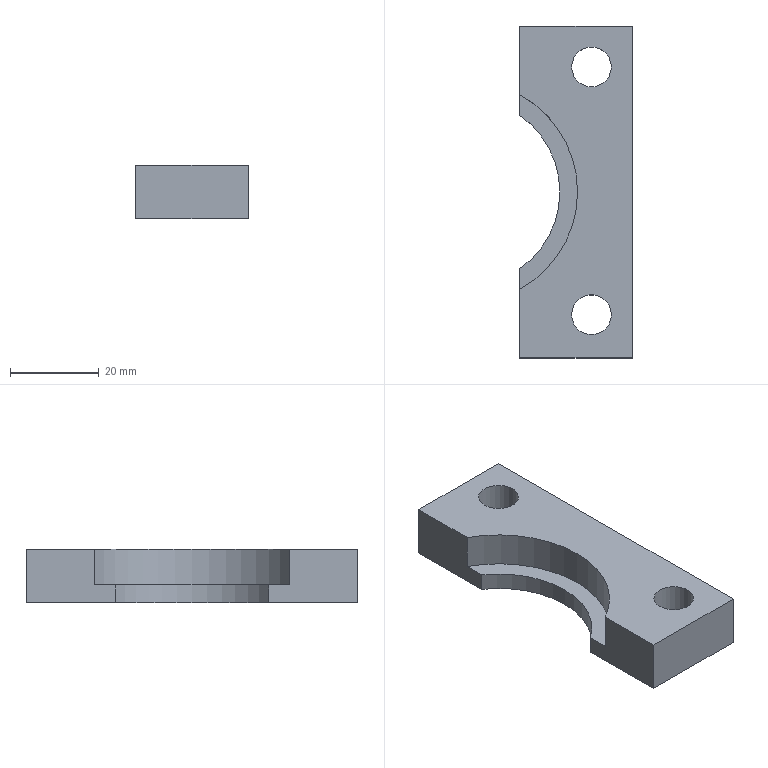Part | NX | features solid 2 | 1 solid | 12 faces | box 25.5 x 75 x 12 mm | volume 17248 mm3 | plane 8 | cylinder 4 | commonest cylinder face diameters 9 x2 42.2 x1 50.2 x1
STEP:
#1=CARTESIAN_POINT('',(772.5,172.5,250.));
#2=VERTEX_POINT('',#1);
#3=CARTESIAN_POINT('',(747.,172.5,250.));
#4=VERTEX_POINT('',#3);
#5=CARTESIAN_POINT('',(772.5,172.5,250.));
#6=DIRECTION('',(-1.,0.,0.));
#7=VECTOR('',#6,1000.);
#8=LINE('',#5,#7);
#9=EDGE_CURVE('',#2,#4,#8,.T.);
#10=ORIENTED_EDGE('',*,*,#9,.T.);
#11=CARTESIAN_POINT('',(747.,172.5,238.));
#12=VERTEX_POINT('',#11);
#13=CARTESIAN_POINT('',(747.,172.5,242.));
#14=DIRECTION('',(0.,0.,1.));
#15=VECTOR('',#14,1000.);
#16=LINE('',#13,#15);
#17=EDGE_CURVE('',#12,#4,#16,.T.);
#18=ORIENTED_EDGE('',*,*,#17,.F.);
#19=CARTESIAN_POINT('',(772.5,172.5,238.));
#20=VERTEX_POINT('',#19);
#21=CARTESIAN_POINT('',(772.5,172.5,238.));
#22=DIRECTION('',(-1.,0.,0.));
#23=VECTOR('',#22,1000.);
#24=LINE('',#21,#23);
#25=EDGE_CURVE('',#20,#12,#24,.T.);
#26=ORIENTED_EDGE('',*,*,#25,.F.);
#27=CARTESIAN_POINT('',(772.5,172.5,242.));
#28=DIRECTION('',(0.,0.,1.));
#29=VECTOR('',#28,1000.);
#30=LINE('',#27,#29);
#31=EDGE_CURVE('',#20,#2,#30,.T.);
#32=ORIENTED_EDGE('',*,*,#31,.T.);
#33=EDGE_LOOP('',(#10,#18,#26,#32));
#34=FACE_BOUND('',#33,.T.);
#35=CARTESIAN_POINT('',(772.5,172.5,242.));
#36=DIRECTION('',(0.,1.,0.));
#37=DIRECTION('',(0.,0.,1.));
#38=AXIS2_PLACEMENT_3D('',#35,#36,#37);
#39=PLANE('',#38);
#40=ADVANCED_FACE('',(#34),#39,.F.);
#41=CARTESIAN_POINT('',(772.5,247.5,250.));
#42=VERTEX_POINT('',#41);
#43=CARTESIAN_POINT('',(772.5,247.5,250.));
#44=DIRECTION('',(0.,-1.,0.));
#45=VECTOR('',#44,1000.);
#46=LINE('',#43,#45);
#47=EDGE_CURVE('',#42,#2,#46,.T.);
#48=ORIENTED_EDGE('',*,*,#47,.T.);
#49=ORIENTED_EDGE('',*,*,#31,.F.);
#50=CARTESIAN_POINT('',(772.5,247.5,238.));
#51=VERTEX_POINT('',#50);
#52=CARTESIAN_POINT('',(772.5,247.5,238.));
#53=DIRECTION('',(0.,-1.,0.));
#54=VECTOR('',#53,1000.);
#55=LINE('',#52,#54);
#56=EDGE_CURVE('',#51,#20,#55,.T.);
#57=ORIENTED_EDGE('',*,*,#56,.F.);
#58=CARTESIAN_POINT('',(772.5,247.5,242.));
#59=DIRECTION('',(0.,0.,1.));
#60=VECTOR('',#59,1000.);
#61=LINE('',#58,#60);
#62=EDGE_CURVE('',#51,#42,#61,.T.);
#63=ORIENTED_EDGE('',*,*,#62,.T.);
#64=EDGE_LOOP('',(#48,#49,#57,#63));
#65=FACE_BOUND('',#64,.T.);
#66=CARTESIAN_POINT('',(772.5,247.5,242.));
#67=DIRECTION('',(-1.,0.,0.));
#68=DIRECTION('',(0.,-1.,0.));
#69=AXIS2_PLACEMENT_3D('',#66,#67,#68);
#70=PLANE('',#69);
#71=ADVANCED_FACE('',(#65),#70,.F.);
#72=CARTESIAN_POINT('',(747.,247.5,250.));
#73=VERTEX_POINT('',#72);
#74=CARTESIAN_POINT('',(747.,247.5,250.));
#75=DIRECTION('',(1.,0.,0.));
#76=VECTOR('',#75,1000.);
#77=LINE('',#74,#76);
#78=EDGE_CURVE('',#73,#42,#77,.T.);
#79=ORIENTED_EDGE('',*,*,#78,.T.);
#80=ORIENTED_EDGE('',*,*,#62,.F.);
#81=CARTESIAN_POINT('',(747.,247.5,238.));
#82=VERTEX_POINT('',#81);
#83=CARTESIAN_POINT('',(747.,247.5,238.));
#84=DIRECTION('',(1.,0.,0.));
#85=VECTOR('',#84,1000.);
#86=LINE('',#83,#85);
#87=EDGE_CURVE('',#82,#51,#86,.T.);
#88=ORIENTED_EDGE('',*,*,#87,.F.);
#89=CARTESIAN_POINT('',(747.,247.5,242.));
#90=DIRECTION('',(0.,0.,1.));
#91=VECTOR('',#90,1000.);
#92=LINE('',#89,#91);
#93=EDGE_CURVE('',#82,#73,#92,.T.);
#94=ORIENTED_EDGE('',*,*,#93,.T.);
#95=EDGE_LOOP('',(#79,#80,#88,#94));
#96=FACE_BOUND('',#95,.T.);
#97=CARTESIAN_POINT('',(747.,247.5,242.));
#98=DIRECTION('',(0.,-1.,0.));
#99=DIRECTION('',(0.,0.,-1.));
#100=AXIS2_PLACEMENT_3D('',#97,#98,#99);
#101=PLANE('',#100);
#102=ADVANCED_FACE('',(#96),#101,.F.);
#103=CARTESIAN_POINT('',(747.,232.046,250.));
#104=VERTEX_POINT('',#103);
#105=CARTESIAN_POINT('',(747.,247.5,250.));
#106=DIRECTION('',(0.,-1.,0.));
#107=VECTOR('',#106,1000.);
#108=LINE('',#105,#107);
#109=EDGE_CURVE('',#73,#104,#108,.T.);
#110=ORIENTED_EDGE('',*,*,#109,.F.);
#111=ORIENTED_EDGE('',*,*,#93,.F.);
#112=CARTESIAN_POINT('',(747.,227.355,238.));
#113=VERTEX_POINT('',#112);
#114=CARTESIAN_POINT('',(747.,247.5,238.));
#115=DIRECTION('',(0.,-1.,0.));
#116=VECTOR('',#115,1000.);
#117=LINE('',#114,#116);
#118=EDGE_CURVE('',#82,#113,#117,.T.);
#119=ORIENTED_EDGE('',*,*,#118,.T.);
#120=CARTESIAN_POINT('',(747.,227.355,242.));
#121=VERTEX_POINT('',#120);
#122=CARTESIAN_POINT('',(747.,227.355,238.));
#123=DIRECTION('',(0.,0.,1.));
#124=VECTOR('',#123,1000.);
#125=LINE('',#122,#124);
#126=EDGE_CURVE('',#113,#121,#125,.T.);
#127=ORIENTED_EDGE('',*,*,#126,.T.);
#128=CARTESIAN_POINT('',(747.,232.046,242.));
#129=VERTEX_POINT('',#128);
#130=CARTESIAN_POINT('',(747.,247.5,242.));
#131=DIRECTION('',(0.,-1.,0.));
#132=VECTOR('',#131,1000.);
#133=LINE('',#130,#132);
#134=EDGE_CURVE('',#129,#121,#133,.T.);
#135=ORIENTED_EDGE('',*,*,#134,.F.);
#136=CARTESIAN_POINT('',(747.,232.046,242.));
#137=DIRECTION('',(0.,0.,1.));
#138=VECTOR('',#137,1000.);
#139=LINE('',#136,#138);
#140=EDGE_CURVE('',#129,#104,#139,.T.);
#141=ORIENTED_EDGE('',*,*,#140,.T.);
#142=EDGE_LOOP('',(#110,#111,#119,#127,#135,#141));
#143=FACE_BOUND('',#142,.T.);
#144=CARTESIAN_POINT('',(747.,247.5,242.));
#145=DIRECTION('',(-1.,0.,0.));
#146=DIRECTION('',(0.,-1.,0.));
#147=AXIS2_PLACEMENT_3D('',#144,#145,#146);
#148=PLANE('',#147);
#149=ADVANCED_FACE('',(#143),#148,.T.);
#150=CARTESIAN_POINT('',(747.,187.954,250.));
#151=VERTEX_POINT('',#150);
#152=CARTESIAN_POINT('',(735.,210.,250.));
#153=DIRECTION('',(0.,0.,1.));
#154=DIRECTION('',(1.,0.,0.));
#155=AXIS2_PLACEMENT_3D('',#152,#153,#154);
#156=CIRCLE('',#155,25.1);
#157=EDGE_CURVE('',#151,#104,#156,.T.);
#158=ORIENTED_EDGE('',*,*,#157,.T.);
#159=ORIENTED_EDGE('',*,*,#140,.F.);
#160=CARTESIAN_POINT('',(747.,187.954,242.));
#161=VERTEX_POINT('',#160);
#162=CARTESIAN_POINT('',(735.,210.,242.));
#163=DIRECTION('',(0.,0.,1.));
#164=DIRECTION('',(1.,0.,0.));
#165=AXIS2_PLACEMENT_3D('',#162,#163,#164);
#166=CIRCLE('',#165,25.1);
#167=EDGE_CURVE('',#161,#129,#166,.T.);
#168=ORIENTED_EDGE('',*,*,#167,.F.);
#169=CARTESIAN_POINT('',(747.,187.954,242.));
#170=DIRECTION('',(0.,0.,1.));
#171=VECTOR('',#170,1000.);
#172=LINE('',#169,#171);
#173=EDGE_CURVE('',#161,#151,#172,.T.);
#174=ORIENTED_EDGE('',*,*,#173,.T.);
#175=EDGE_LOOP('',(#158,#159,#168,#174));
#176=FACE_BOUND('',#175,.T.);
#177=CARTESIAN_POINT('',(735.,210.,242.));
#178=DIRECTION('',(0.,0.,1.));
#179=DIRECTION('',(1.,0.,0.));
#180=AXIS2_PLACEMENT_3D('',#177,#178,#179);
#181=CYLINDRICAL_SURFACE('',#180,25.1);
#182=ADVANCED_FACE('',(#176),#181,.F.);
#183=CARTESIAN_POINT('',(747.,192.645,250.));
#184=DIRECTION('',(0.,-1.,0.));
#185=VECTOR('',#184,1000.);
#186=LINE('',#183,#185);
#187=EDGE_CURVE('',#151,#4,#186,.T.);
#188=ORIENTED_EDGE('',*,*,#187,.F.);
#189=ORIENTED_EDGE('',*,*,#173,.F.);
#190=CARTESIAN_POINT('',(747.,192.645,242.));
#191=VERTEX_POINT('',#190);
#192=CARTESIAN_POINT('',(747.,192.645,242.));
#193=DIRECTION('',(0.,-1.,0.));
#194=VECTOR('',#193,1000.);
#195=LINE('',#192,#194);
#196=EDGE_CURVE('',#191,#161,#195,.T.);
#197=ORIENTED_EDGE('',*,*,#196,.F.);
#198=CARTESIAN_POINT('',(747.,192.645,238.));
#199=VERTEX_POINT('',#198);
#200=CARTESIAN_POINT('',(747.,192.645,238.));
#201=DIRECTION('',(0.,0.,1.));
#202=VECTOR('',#201,1000.);
#203=LINE('',#200,#202);
#204=EDGE_CURVE('',#199,#191,#203,.T.);
#205=ORIENTED_EDGE('',*,*,#204,.F.);
#206=CARTESIAN_POINT('',(747.,192.645,238.));
#207=DIRECTION('',(0.,-1.,0.));
#208=VECTOR('',#207,1000.);
#209=LINE('',#206,#208);
#210=EDGE_CURVE('',#199,#12,#209,.T.);
#211=ORIENTED_EDGE('',*,*,#210,.T.);
#212=ORIENTED_EDGE('',*,*,#17,.T.);
#213=EDGE_LOOP('',(#188,#189,#197,#205,#211,#212));
#214=FACE_BOUND('',#213,.T.);
#215=CARTESIAN_POINT('',(747.,192.645,242.));
#216=DIRECTION('',(-1.,0.,0.));
#217=DIRECTION('',(0.,-1.,0.));
#218=AXIS2_PLACEMENT_3D('',#215,#216,#217);
#219=PLANE('',#218);
#220=ADVANCED_FACE('',(#214),#219,.T.);
#221=CARTESIAN_POINT('',(767.75,238.25,250.));
#222=VERTEX_POINT('',#221);
#223=CARTESIAN_POINT('',(763.25,238.25,250.));
#224=DIRECTION('',(0.,0.,1.));
#225=DIRECTION('',(1.,0.,0.));
#226=AXIS2_PLACEMENT_3D('',#223,#224,#225);
#227=CIRCLE('',#226,4.5);
#228=EDGE_CURVE('',#222,#222,#227,.T.);
#229=ORIENTED_EDGE('',*,*,#228,.F.);
#230=EDGE_LOOP('',(#229));
#231=FACE_BOUND('',#230,.T.);
#232=CARTESIAN_POINT('',(767.75,182.25,250.));
#233=VERTEX_POINT('',#232);
#234=CARTESIAN_POINT('',(763.25,182.25,250.));
#235=DIRECTION('',(0.,0.,1.));
#236=DIRECTION('',(1.,0.,0.));
#237=AXIS2_PLACEMENT_3D('',#234,#235,#236);
#238=CIRCLE('',#237,4.5);
#239=EDGE_CURVE('',#233,#233,#238,.T.);
#240=ORIENTED_EDGE('',*,*,#239,.F.);
#241=EDGE_LOOP('',(#240));
#242=FACE_BOUND('',#241,.T.);
#243=ORIENTED_EDGE('',*,*,#9,.F.);
#244=ORIENTED_EDGE('',*,*,#47,.F.);
#245=ORIENTED_EDGE('',*,*,#78,.F.);
#246=ORIENTED_EDGE('',*,*,#109,.T.);
#247=ORIENTED_EDGE('',*,*,#157,.F.);
#248=ORIENTED_EDGE('',*,*,#187,.T.);
#249=EDGE_LOOP('',(#243,#244,#245,#246,#247,#248));
#250=FACE_BOUND('',#249,.T.);
#251=CARTESIAN_POINT('',(757.683,216.25,250.));
#252=DIRECTION('',(0.,0.,1.));
#253=DIRECTION('',(1.,0.,0.));
#254=AXIS2_PLACEMENT_3D('',#251,#252,#253);
#255=PLANE('',#254);
#256=ADVANCED_FACE('',(#231,#242,#250),#255,.T.);
#257=ORIENTED_EDGE('',*,*,#239,.T.);
#258=EDGE_LOOP('',(#257));
#259=FACE_BOUND('',#258,.T.);
#260=CARTESIAN_POINT('',(767.75,182.25,238.));
#261=VERTEX_POINT('',#260);
#262=CARTESIAN_POINT('',(763.25,182.25,238.));
#263=DIRECTION('',(0.,0.,1.));
#264=DIRECTION('',(1.,0.,0.));
#265=AXIS2_PLACEMENT_3D('',#262,#263,#264);
#266=CIRCLE('',#265,4.5);
#267=EDGE_CURVE('',#261,#261,#266,.T.);
#268=ORIENTED_EDGE('',*,*,#267,.F.);
#269=EDGE_LOOP('',(#268));
#270=FACE_BOUND('',#269,.T.);
#271=CARTESIAN_POINT('',(763.25,182.25,242.));
#272=DIRECTION('',(0.,0.,1.));
#273=DIRECTION('',(1.,0.,0.));
#274=AXIS2_PLACEMENT_3D('',#271,#272,#273);
#275=CYLINDRICAL_SURFACE('',#274,4.5);
#276=ADVANCED_FACE('',(#259,#270),#275,.F.);
#277=ORIENTED_EDGE('',*,*,#228,.T.);
#278=EDGE_LOOP('',(#277));
#279=FACE_BOUND('',#278,.T.);
#280=CARTESIAN_POINT('',(767.75,238.25,238.));
#281=VERTEX_POINT('',#280);
#282=CARTESIAN_POINT('',(763.25,238.25,238.));
#283=DIRECTION('',(0.,0.,1.));
#284=DIRECTION('',(1.,0.,0.));
#285=AXIS2_PLACEMENT_3D('',#282,#283,#284);
#286=CIRCLE('',#285,4.5);
#287=EDGE_CURVE('',#281,#281,#286,.T.);
#288=ORIENTED_EDGE('',*,*,#287,.F.);
#289=EDGE_LOOP('',(#288));
#290=FACE_BOUND('',#289,.T.);
#291=CARTESIAN_POINT('',(763.25,238.25,242.));
#292=DIRECTION('',(0.,0.,1.));
#293=DIRECTION('',(1.,0.,0.));
#294=AXIS2_PLACEMENT_3D('',#291,#292,#293);
#295=CYLINDRICAL_SURFACE('',#294,4.5);
#296=ADVANCED_FACE('',(#279,#290),#295,.F.);
#297=ORIENTED_EDGE('',*,*,#196,.T.);
#298=ORIENTED_EDGE('',*,*,#167,.T.);
#299=ORIENTED_EDGE('',*,*,#134,.T.);
#300=CARTESIAN_POINT('',(735.,210.,242.));
#301=DIRECTION('',(0.,0.,1.));
#302=DIRECTION('',(1.,0.,0.));
#303=AXIS2_PLACEMENT_3D('',#300,#301,#302);
#304=CIRCLE('',#303,21.1);
#305=EDGE_CURVE('',#191,#121,#304,.T.);
#306=ORIENTED_EDGE('',*,*,#305,.F.);
#307=EDGE_LOOP('',(#297,#298,#299,#306));
#308=FACE_BOUND('',#307,.T.);
#309=CARTESIAN_POINT('',(735.,210.,242.));
#310=DIRECTION('',(0.,0.,1.));
#311=DIRECTION('',(1.,0.,0.));
#312=AXIS2_PLACEMENT_3D('',#309,#310,#311);
#313=PLANE('',#312);
#314=ADVANCED_FACE('',(#308),#313,.T.);
#315=ORIENTED_EDGE('',*,*,#267,.T.);
#316=EDGE_LOOP('',(#315));
#317=FACE_BOUND('',#316,.T.);
#318=ORIENTED_EDGE('',*,*,#287,.T.);
#319=EDGE_LOOP('',(#318));
#320=FACE_BOUND('',#319,.T.);
#321=ORIENTED_EDGE('',*,*,#87,.T.);
#322=ORIENTED_EDGE('',*,*,#56,.T.);
#323=ORIENTED_EDGE('',*,*,#25,.T.);
#324=ORIENTED_EDGE('',*,*,#210,.F.);
#325=CARTESIAN_POINT('',(735.,210.,238.));
#326=DIRECTION('',(0.,0.,1.));
#327=DIRECTION('',(1.,0.,0.));
#328=AXIS2_PLACEMENT_3D('',#325,#326,#327);
#329=CIRCLE('',#328,21.1);
#330=EDGE_CURVE('',#199,#113,#329,.T.);
#331=ORIENTED_EDGE('',*,*,#330,.T.);
#332=ORIENTED_EDGE('',*,*,#118,.F.);
#333=EDGE_LOOP('',(#321,#322,#323,#324,#331,#332));
#334=FACE_BOUND('',#333,.T.);
#335=CARTESIAN_POINT('',(735.,210.,238.));
#336=DIRECTION('',(0.,0.,1.));
#337=DIRECTION('',(1.,0.,0.));
#338=AXIS2_PLACEMENT_3D('',#335,#336,#337);
#339=PLANE('',#338);
#340=ADVANCED_FACE('',(#317,#320,#334),#339,.F.);
#341=ORIENTED_EDGE('',*,*,#305,.T.);
#342=ORIENTED_EDGE('',*,*,#126,.F.);
#343=ORIENTED_EDGE('',*,*,#330,.F.);
#344=ORIENTED_EDGE('',*,*,#204,.T.);
#345=EDGE_LOOP('',(#341,#342,#343,#344));
#346=FACE_BOUND('',#345,.T.);
#347=CARTESIAN_POINT('',(735.,210.,238.));
#348=DIRECTION('',(0.,0.,1.));
#349=DIRECTION('',(1.,0.,0.));
#350=AXIS2_PLACEMENT_3D('',#347,#348,#349);
#351=CYLINDRICAL_SURFACE('',#350,21.1);
#352=ADVANCED_FACE('',(#346),#351,.F.);
#353=CLOSED_SHELL('',(#40,#71,#102,#149,#182,#220,#256,#276,#296,#314,#340,#352));
#354=MANIFOLD_SOLID_BREP('',#353);
#355=(LENGTH_UNIT()NAMED_UNIT(*)SI_UNIT(.MILLI.,.METRE.));
#356=UNCERTAINTY_MEASURE_WITH_UNIT(LENGTH_MEASURE(0.00001),#355,'','');
#357=(NAMED_UNIT(*)PLANE_ANGLE_UNIT()SI_UNIT($,.RADIAN.));
#358=(NAMED_UNIT(*)SI_UNIT($,.STERADIAN.)SOLID_ANGLE_UNIT());
#359=(GEOMETRIC_REPRESENTATION_CONTEXT(3)GLOBAL_UNCERTAINTY_ASSIGNED_CONTEXT((#356))GLOBAL_UNIT_ASSIGNED_CONTEXT((#355,#357,#358))REPRESENTATION_CONTEXT('',''));
#360=ADVANCED_BREP_SHAPE_REPRESENTATION('',(#354),#359);